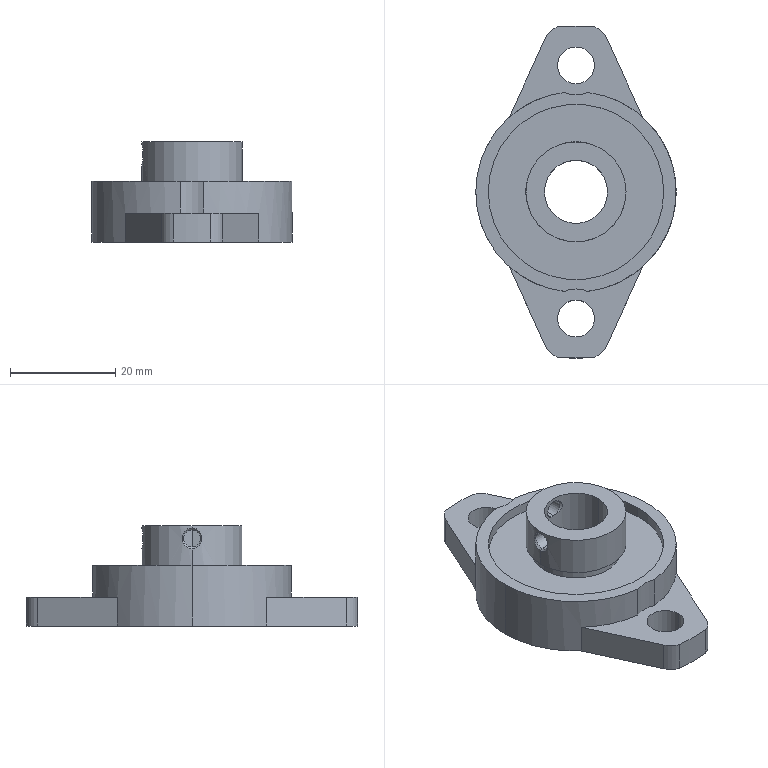Part | STEP file | 0232_Z_HBRS12_1 | 1 solid | 52 faces | box 38 x 63 x 19 mm | volume 12458 mm3 | cylinder 29 | plane 13 | cone 8 | spline 2 | commonest cylinder face diameters 3.242 x4 7 x4 7.6 x4 33.25 x4 38 x3 11.2 x2